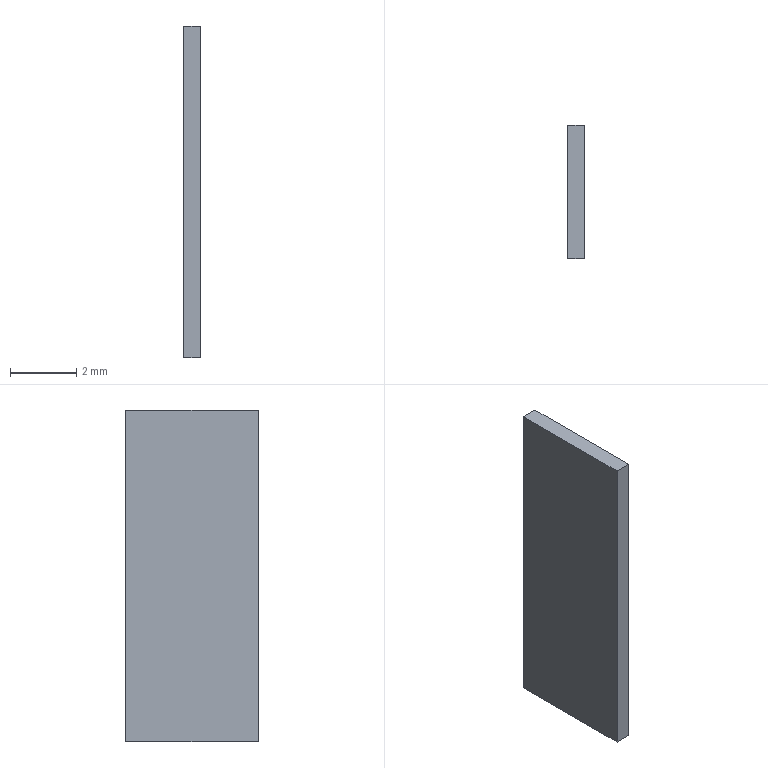Part | SolidWorks | features BaseBody 1 | 1 solid | 77 faces | box 0.5 x 4 x 10 mm | volume 19.291 mm3 | plane 41 | spline 36